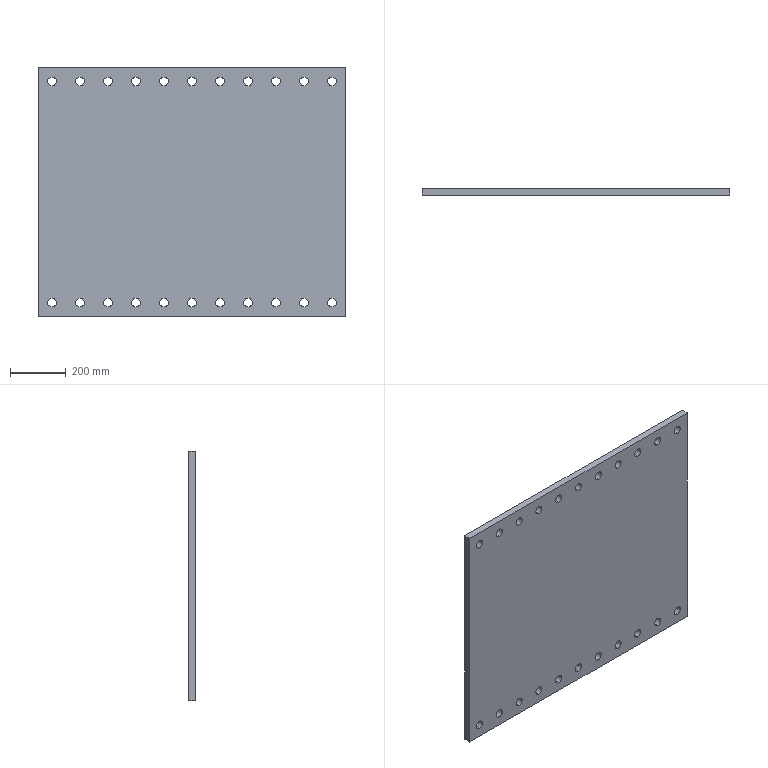Part | SolidWorks | features FlatPattern 1, SMBaseFlange 1, SheetMetal 1 | 1 solid | 50 faces | box 1100 x 25 x 890 mm | volume 24059878 mm3 | cylinder 44 | plane 6 | commonest cylinder face diameters 31 x44